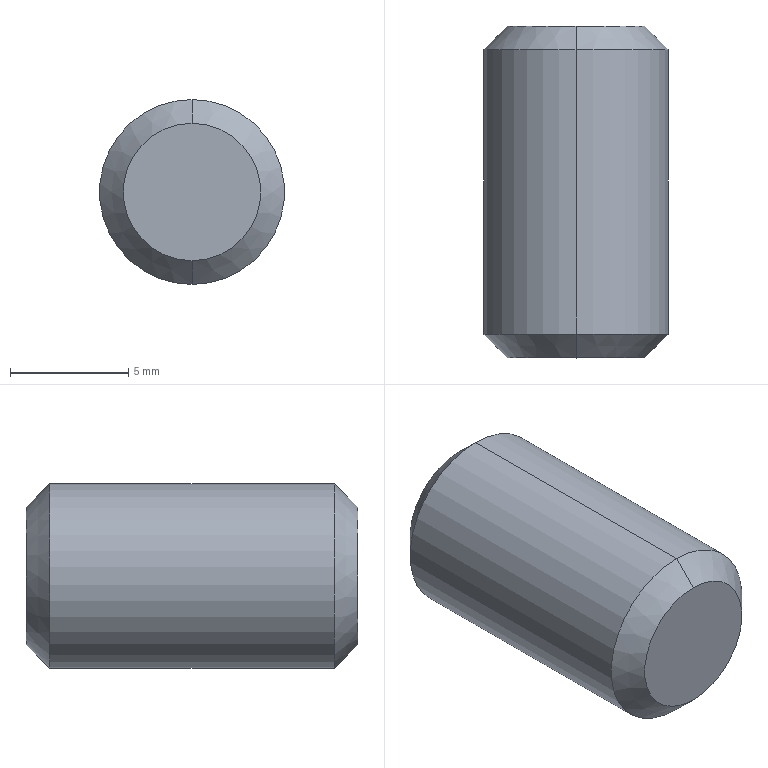Part | STEP file | Ngam kep 17 | 1 solid | 12 faces | box 7.8 x 14 x 7.8 mm | volume 557.349 mm3 | cone 6 | cylinder 4 | plane 2 | commonest cylinder face diameters 3.3 x2 7.8 x2
STEP:
#1=CARTESIAN_POINT('',(0.,0.,0.));
#2=DIRECTION('',(0.,0.,1.));
#3=DIRECTION('',(1.,0.,0.));
#4=AXIS2_PLACEMENT_3D('',#1,#2,#3);
#5=CARTESIAN_POINT('',(0.,14.,2.9));
#6=VERTEX_POINT('',#5);
#7=CARTESIAN_POINT('',(0.,14.,-2.9));
#8=VERTEX_POINT('',#7);
#9=CARTESIAN_POINT('',(0.,14.,0.));
#10=DIRECTION('',(0.,1.,0.));
#11=DIRECTION('',(0.,0.,1.));
#12=AXIS2_PLACEMENT_3D('',#9,#10,#11);
#13=CIRCLE('',#12,2.9);
#14=CARTESIAN_POINT('',(0.,14.,0.));
#15=DIRECTION('',(0.,-1.,0.));
#16=DIRECTION('',(0.,0.,-1.));
#17=AXIS2_PLACEMENT_3D('',#14,#15,#16);
#18=CONICAL_SURFACE('',#17,2.9,0.7854);
#19=CARTESIAN_POINT('',(3.142,0.));
#20=DIRECTION('',(-1.,0.));
#21=VECTOR('',#20,1.);
#22=LINE('',#19,#21);
#23=(GEOMETRIC_REPRESENTATION_CONTEXT(2)PARAMETRIC_REPRESENTATION_CONTEXT()REPRESENTATION_CONTEXT('',''));
#24=DEFINITIONAL_REPRESENTATION('',(#22),#23);
#25=PCURVE('',#18,#24);
#26=CARTESIAN_POINT('',(0.,14.,0.));
#27=DIRECTION('',(0.,1.,0.));
#28=DIRECTION('',(0.,0.,1.));
#29=AXIS2_PLACEMENT_3D('',#26,#27,#28);
#30=PLANE('',#29);
#31=CARTESIAN_POINT('',(0.,0.));
#32=DIRECTION('',(1.,0.));
#33=AXIS2_PLACEMENT_2D('',#31,#32);
#34=CIRCLE('',#33,2.9);
#35=(GEOMETRIC_REPRESENTATION_CONTEXT(2)PARAMETRIC_REPRESENTATION_CONTEXT()REPRESENTATION_CONTEXT('',''));
#36=DEFINITIONAL_REPRESENTATION('',(#34),#35);
#37=PCURVE('',#30,#36);
#38=SURFACE_CURVE('',#13,(#25,#37),.PCURVE_S1.);
#39=EDGE_CURVE('',#6,#8,#38,.T.);
#40=ORIENTED_EDGE('',*,*,#39,.F.);
#41=CARTESIAN_POINT('',(0.,13.,3.9));
#42=VERTEX_POINT('',#41);
#43=CARTESIAN_POINT('',(0.,14.,2.9));
#44=DIRECTION('',(0.,-0.7071,0.7071));
#45=VECTOR('',#44,1.);
#46=LINE('',#43,#45);
#47=CARTESIAN_POINT('',(3.142,0.));
#48=DIRECTION('',(0.,1.));
#49=VECTOR('',#48,1.);
#50=LINE('',#47,#49);
#51=(GEOMETRIC_REPRESENTATION_CONTEXT(2)PARAMETRIC_REPRESENTATION_CONTEXT()REPRESENTATION_CONTEXT('',''));
#52=DEFINITIONAL_REPRESENTATION('',(#50),#51);
#53=PCURVE('',#18,#52);
#54=CARTESIAN_POINT('',(0.,14.,0.));
#55=DIRECTION('',(0.,-1.,0.));
#56=DIRECTION('',(0.,0.,-1.));
#57=AXIS2_PLACEMENT_3D('',#54,#55,#56);
#58=CONICAL_SURFACE('',#57,2.9,0.7854);
#59=CARTESIAN_POINT('',(3.142,0.));
#60=DIRECTION('',(0.,1.));
#61=VECTOR('',#60,1.);
#62=LINE('',#59,#61);
#63=(GEOMETRIC_REPRESENTATION_CONTEXT(2)PARAMETRIC_REPRESENTATION_CONTEXT()REPRESENTATION_CONTEXT('',''));
#64=DEFINITIONAL_REPRESENTATION('',(#62),#63);
#65=PCURVE('',#58,#64);
#66=SURFACE_CURVE('',#46,(#53,#65),.PCURVE_S1.);
#67=EDGE_CURVE('',#6,#42,#66,.T.);
#68=ORIENTED_EDGE('',*,*,#67,.T.);
#69=CARTESIAN_POINT('',(0.,13.,-3.9));
#70=VERTEX_POINT('',#69);
#71=CARTESIAN_POINT('',(0.,13.,0.));
#72=DIRECTION('',(0.,-1.,0.));
#73=DIRECTION('',(0.,0.,1.));
#74=AXIS2_PLACEMENT_3D('',#71,#72,#73);
#75=CIRCLE('',#74,3.9);
#76=CARTESIAN_POINT('',(-3.142,1.));
#77=DIRECTION('',(1.,0.));
#78=VECTOR('',#77,1.);
#79=LINE('',#76,#78);
#80=(GEOMETRIC_REPRESENTATION_CONTEXT(2)PARAMETRIC_REPRESENTATION_CONTEXT()REPRESENTATION_CONTEXT('',''));
#81=DEFINITIONAL_REPRESENTATION('',(#79),#80);
#82=PCURVE('',#18,#81);
#83=CARTESIAN_POINT('',(0.,14.,0.));
#84=DIRECTION('',(0.,-1.,0.));
#85=DIRECTION('',(0.,0.,-1.));
#86=AXIS2_PLACEMENT_3D('',#83,#84,#85);
#87=CYLINDRICAL_SURFACE('',#86,3.9);
#88=CARTESIAN_POINT('',(-3.142,1.));
#89=DIRECTION('',(1.,0.));
#90=VECTOR('',#89,1.);
#91=LINE('',#88,#90);
#92=(GEOMETRIC_REPRESENTATION_CONTEXT(2)PARAMETRIC_REPRESENTATION_CONTEXT()REPRESENTATION_CONTEXT('',''));
#93=DEFINITIONAL_REPRESENTATION('',(#91),#92);
#94=PCURVE('',#87,#93);
#95=SURFACE_CURVE('',#75,(#82,#94),.PCURVE_S1.);
#96=EDGE_CURVE('',#70,#42,#95,.T.);
#97=ORIENTED_EDGE('',*,*,#96,.F.);
#98=CARTESIAN_POINT('',(0.,14.,-2.9));
#99=DIRECTION('',(0.,-0.7071,-0.7071));
#100=VECTOR('',#99,1.);
#101=LINE('',#98,#100);
#102=CARTESIAN_POINT('',(0.,0.));
#103=DIRECTION('',(0.,1.));
#104=VECTOR('',#103,1.);
#105=LINE('',#102,#104);
#106=(GEOMETRIC_REPRESENTATION_CONTEXT(2)PARAMETRIC_REPRESENTATION_CONTEXT()REPRESENTATION_CONTEXT('',''));
#107=DEFINITIONAL_REPRESENTATION('',(#105),#106);
#108=PCURVE('',#18,#107);
#109=CARTESIAN_POINT('',(6.283,0.));
#110=DIRECTION('',(0.,1.));
#111=VECTOR('',#110,1.);
#112=LINE('',#109,#111);
#113=(GEOMETRIC_REPRESENTATION_CONTEXT(2)PARAMETRIC_REPRESENTATION_CONTEXT()REPRESENTATION_CONTEXT('',''));
#114=DEFINITIONAL_REPRESENTATION('',(#112),#113);
#115=PCURVE('',#58,#114);
#116=SURFACE_CURVE('',#101,(#108,#115),.PCURVE_S1.);
#117=EDGE_CURVE('',#8,#70,#116,.T.);
#118=ORIENTED_EDGE('',*,*,#117,.F.);
#119=EDGE_LOOP('',(#40,#68,#97,#118));
#120=FACE_BOUND('',#119,.T.);
#121=ADVANCED_FACE('',(#120),#18,.T.);
#122=CARTESIAN_POINT('',(0.,0.,-2.9));
#123=VERTEX_POINT('',#122);
#124=CARTESIAN_POINT('',(0.,0.,2.9));
#125=VERTEX_POINT('',#124);
#126=CARTESIAN_POINT('',(0.,0.,0.));
#127=DIRECTION('',(0.,-1.,0.));
#128=DIRECTION('',(0.,0.,1.));
#129=AXIS2_PLACEMENT_3D('',#126,#127,#128);
#130=CIRCLE('',#129,2.9);
#131=CARTESIAN_POINT('',(0.,1.,0.));
#132=DIRECTION('',(0.,1.,0.));
#133=DIRECTION('',(0.,0.,1.));
#134=AXIS2_PLACEMENT_3D('',#131,#132,#133);
#135=CONICAL_SURFACE('',#134,3.9,0.7854);
#136=CARTESIAN_POINT('',(6.283,-1.));
#137=DIRECTION('',(-1.,0.));
#138=VECTOR('',#137,1.);
#139=LINE('',#136,#138);
#140=(GEOMETRIC_REPRESENTATION_CONTEXT(2)PARAMETRIC_REPRESENTATION_CONTEXT()REPRESENTATION_CONTEXT('',''));
#141=DEFINITIONAL_REPRESENTATION('',(#139),#140);
#142=PCURVE('',#135,#141);
#143=CARTESIAN_POINT('',(0.,0.,0.));
#144=DIRECTION('',(0.,1.,0.));
#145=DIRECTION('',(0.,0.,1.));
#146=AXIS2_PLACEMENT_3D('',#143,#144,#145);
#147=PLANE('',#146);
#148=CARTESIAN_POINT('',(2.9,0.));
#149=CARTESIAN_POINT('',(2.9,-5.023));
#150=CARTESIAN_POINT('',(-1.45,-2.511));
#151=CARTESIAN_POINT('',(-5.8,0.));
#152=CARTESIAN_POINT('',(-1.45,2.511));
#153=CARTESIAN_POINT('',(2.9,5.023));
#154=CARTESIAN_POINT('',(2.9,0.));
#155=(BOUNDED_CURVE()B_SPLINE_CURVE(2,(#148,#149,#150,#151,#152,#153,#154),.UNSPECIFIED.,.T.,.F.)B_SPLINE_CURVE_WITH_KNOTS((1,2,2,2,2,1),(-2.094,0.,2.094,4.189,6.283,8.378),.UNSPECIFIED.)CURVE()GEOMETRIC_REPRESENTATION_ITEM()RATIONAL_B_SPLINE_CURVE((1.,0.5,1.,0.5,1.,0.5,1.))REPRESENTATION_ITEM(''));
#156=(GEOMETRIC_REPRESENTATION_CONTEXT(2)PARAMETRIC_REPRESENTATION_CONTEXT()REPRESENTATION_CONTEXT('',''));
#157=DEFINITIONAL_REPRESENTATION('',(#155),#156);
#158=PCURVE('',#147,#157);
#159=SURFACE_CURVE('',#130,(#142,#158),.PCURVE_S1.);
#160=EDGE_CURVE('',#123,#125,#159,.T.);
#161=ORIENTED_EDGE('',*,*,#160,.F.);
#162=CARTESIAN_POINT('',(0.,1.,-3.9));
#163=VERTEX_POINT('',#162);
#164=CARTESIAN_POINT('',(0.,1.,-3.9));
#165=DIRECTION('',(0.,0.7071,-0.7071));
#166=VECTOR('',#165,1.);
#167=LINE('',#164,#166);
#168=CARTESIAN_POINT('',(3.142,0.));
#169=DIRECTION('',(0.,1.));
#170=VECTOR('',#169,1.);
#171=LINE('',#168,#170);
#172=(GEOMETRIC_REPRESENTATION_CONTEXT(2)PARAMETRIC_REPRESENTATION_CONTEXT()REPRESENTATION_CONTEXT('',''));
#173=DEFINITIONAL_REPRESENTATION('',(#171),#172);
#174=PCURVE('',#135,#173);
#175=CARTESIAN_POINT('',(0.,1.,0.));
#176=DIRECTION('',(0.,1.,0.));
#177=DIRECTION('',(0.,0.,1.));
#178=AXIS2_PLACEMENT_3D('',#175,#176,#177);
#179=CONICAL_SURFACE('',#178,3.9,0.7854);
#180=CARTESIAN_POINT('',(3.142,0.));
#181=DIRECTION('',(0.,1.));
#182=VECTOR('',#181,1.);
#183=LINE('',#180,#182);
#184=(GEOMETRIC_REPRESENTATION_CONTEXT(2)PARAMETRIC_REPRESENTATION_CONTEXT()REPRESENTATION_CONTEXT('',''));
#185=DEFINITIONAL_REPRESENTATION('',(#183),#184);
#186=PCURVE('',#179,#185);
#187=SURFACE_CURVE('',#167,(#174,#186),.PCURVE_S1.);
#188=EDGE_CURVE('',#123,#163,#187,.T.);
#189=ORIENTED_EDGE('',*,*,#188,.T.);
#190=CARTESIAN_POINT('',(0.,1.,3.9));
#191=VERTEX_POINT('',#190);
#192=CARTESIAN_POINT('',(0.,1.,0.));
#193=DIRECTION('',(0.,1.,0.));
#194=DIRECTION('',(0.,0.,1.));
#195=AXIS2_PLACEMENT_3D('',#192,#193,#194);
#196=CIRCLE('',#195,3.9);
#197=CARTESIAN_POINT('',(0.,0.));
#198=DIRECTION('',(1.,0.));
#199=VECTOR('',#198,1.);
#200=LINE('',#197,#199);
#201=(GEOMETRIC_REPRESENTATION_CONTEXT(2)PARAMETRIC_REPRESENTATION_CONTEXT()REPRESENTATION_CONTEXT('',''));
#202=DEFINITIONAL_REPRESENTATION('',(#200),#201);
#203=PCURVE('',#135,#202);
#204=CARTESIAN_POINT('',(3.142,13.));
#205=DIRECTION('',(-1.,0.));
#206=VECTOR('',#205,1.);
#207=LINE('',#204,#206);
#208=(GEOMETRIC_REPRESENTATION_CONTEXT(2)PARAMETRIC_REPRESENTATION_CONTEXT()REPRESENTATION_CONTEXT('',''));
#209=DEFINITIONAL_REPRESENTATION('',(#207),#208);
#210=PCURVE('',#87,#209);
#211=SURFACE_CURVE('',#196,(#203,#210),.PCURVE_S1.);
#212=EDGE_CURVE('',#191,#163,#211,.T.);
#213=ORIENTED_EDGE('',*,*,#212,.F.);
#214=CARTESIAN_POINT('',(0.,1.,3.9));
#215=DIRECTION('',(0.,0.7071,0.7071));
#216=VECTOR('',#215,1.);
#217=LINE('',#214,#216);
#218=CARTESIAN_POINT('',(0.,0.));
#219=DIRECTION('',(0.,1.));
#220=VECTOR('',#219,1.);
#221=LINE('',#218,#220);
#222=(GEOMETRIC_REPRESENTATION_CONTEXT(2)PARAMETRIC_REPRESENTATION_CONTEXT()REPRESENTATION_CONTEXT('',''));
#223=DEFINITIONAL_REPRESENTATION('',(#221),#222);
#224=PCURVE('',#135,#223);
#225=CARTESIAN_POINT('',(6.283,0.));
#226=DIRECTION('',(0.,1.));
#227=VECTOR('',#226,1.);
#228=LINE('',#225,#227);
#229=(GEOMETRIC_REPRESENTATION_CONTEXT(2)PARAMETRIC_REPRESENTATION_CONTEXT()REPRESENTATION_CONTEXT('',''));
#230=DEFINITIONAL_REPRESENTATION('',(#228),#229);
#231=PCURVE('',#179,#230);
#232=SURFACE_CURVE('',#217,(#224,#231),.PCURVE_S1.);
#233=EDGE_CURVE('',#125,#191,#232,.T.);
#234=ORIENTED_EDGE('',*,*,#233,.F.);
#235=EDGE_LOOP('',(#161,#189,#213,#234));
#236=FACE_BOUND('',#235,.T.);
#237=ADVANCED_FACE('',(#236),#135,.T.);
#238=CARTESIAN_POINT('',(0.,3.9,1.65));
#239=VERTEX_POINT('',#238);
#240=CARTESIAN_POINT('',(0.,14.,1.65));
#241=VERTEX_POINT('',#240);
#242=CARTESIAN_POINT('',(0.,14.,1.65));
#243=DIRECTION('',(0.,1.,0.));
#244=VECTOR('',#243,1.);
#245=LINE('',#242,#244);
#246=CARTESIAN_POINT('',(0.,14.,0.));
#247=DIRECTION('',(0.,1.,0.));
#248=DIRECTION('',(0.,0.,1.));
#249=AXIS2_PLACEMENT_3D('',#246,#247,#248);
#250=CYLINDRICAL_SURFACE('',#249,1.65);
#251=CARTESIAN_POINT('',(6.283,0.));
#252=DIRECTION('',(0.,1.));
#253=VECTOR('',#252,1.);
#254=LINE('',#251,#253);
#255=(GEOMETRIC_REPRESENTATION_CONTEXT(2)PARAMETRIC_REPRESENTATION_CONTEXT()REPRESENTATION_CONTEXT('',''));
#256=DEFINITIONAL_REPRESENTATION('',(#254),#255);
#257=PCURVE('',#250,#256);
#258=CARTESIAN_POINT('',(0.,14.,0.));
#259=DIRECTION('',(0.,1.,0.));
#260=DIRECTION('',(0.,0.,1.));
#261=AXIS2_PLACEMENT_3D('',#258,#259,#260);
#262=CYLINDRICAL_SURFACE('',#261,1.65);
#263=CARTESIAN_POINT('',(0.,0.));
#264=DIRECTION('',(0.,1.));
#265=VECTOR('',#264,1.);
#266=LINE('',#263,#265);
#267=(GEOMETRIC_REPRESENTATION_CONTEXT(2)PARAMETRIC_REPRESENTATION_CONTEXT()REPRESENTATION_CONTEXT('',''));
#268=DEFINITIONAL_REPRESENTATION('',(#266),#267);
#269=PCURVE('',#262,#268);
#270=SURFACE_CURVE('',#245,(#257,#269),.PCURVE_S1.);
#271=EDGE_CURVE('',#239,#241,#270,.T.);
#272=ORIENTED_EDGE('',*,*,#271,.T.);
#273=CARTESIAN_POINT('',(0.,14.,-1.65));
#274=VERTEX_POINT('',#273);
#275=CARTESIAN_POINT('',(0.,14.,0.));
#276=DIRECTION('',(0.,1.,0.));
#277=DIRECTION('',(0.,0.,1.));
#278=AXIS2_PLACEMENT_3D('',#275,#276,#277);
#279=CIRCLE('',#278,1.65);
#280=CARTESIAN_POINT('',(0.,0.));
#281=DIRECTION('',(1.,0.));
#282=VECTOR('',#281,1.);
#283=LINE('',#280,#282);
#284=(GEOMETRIC_REPRESENTATION_CONTEXT(2)PARAMETRIC_REPRESENTATION_CONTEXT()REPRESENTATION_CONTEXT('',''));
#285=DEFINITIONAL_REPRESENTATION('',(#283),#284);
#286=PCURVE('',#250,#285);
#287=CARTESIAN_POINT('',(0.,0.));
#288=DIRECTION('',(1.,0.));
#289=AXIS2_PLACEMENT_2D('',#287,#288);
#290=CIRCLE('',#289,1.65);
#291=(GEOMETRIC_REPRESENTATION_CONTEXT(2)PARAMETRIC_REPRESENTATION_CONTEXT()REPRESENTATION_CONTEXT('',''));
#292=DEFINITIONAL_REPRESENTATION('',(#290),#291);
#293=PCURVE('',#30,#292);
#294=SURFACE_CURVE('',#279,(#286,#293),.PCURVE_S1.);
#295=EDGE_CURVE('',#274,#241,#294,.T.);
#296=ORIENTED_EDGE('',*,*,#295,.F.);
#297=CARTESIAN_POINT('',(0.,3.9,-1.65));
#298=VERTEX_POINT('',#297);
#299=CARTESIAN_POINT('',(0.,14.,-1.65));
#300=DIRECTION('',(0.,1.,0.));
#301=VECTOR('',#300,1.);
#302=LINE('',#299,#301);
#303=CARTESIAN_POINT('',(3.142,0.));
#304=DIRECTION('',(0.,1.));
#305=VECTOR('',#304,1.);
#306=LINE('',#303,#305);
#307=(GEOMETRIC_REPRESENTATION_CONTEXT(2)PARAMETRIC_REPRESENTATION_CONTEXT()REPRESENTATION_CONTEXT('',''));
#308=DEFINITIONAL_REPRESENTATION('',(#306),#307);
#309=PCURVE('',#250,#308);
#310=CARTESIAN_POINT('',(3.142,0.));
#311=DIRECTION('',(0.,1.));
#312=VECTOR('',#311,1.);
#313=LINE('',#310,#312);
#314=(GEOMETRIC_REPRESENTATION_CONTEXT(2)PARAMETRIC_REPRESENTATION_CONTEXT()REPRESENTATION_CONTEXT('',''));
#315=DEFINITIONAL_REPRESENTATION('',(#313),#314);
#316=PCURVE('',#262,#315);
#317=SURFACE_CURVE('',#302,(#309,#316),.PCURVE_S1.);
#318=EDGE_CURVE('',#298,#274,#317,.T.);
#319=ORIENTED_EDGE('',*,*,#318,.F.);
#320=CARTESIAN_POINT('',(0.,3.9,0.));
#321=DIRECTION('',(0.,1.,0.));
#322=DIRECTION('',(0.,0.,1.));
#323=AXIS2_PLACEMENT_3D('',#320,#321,#322);
#324=CIRCLE('',#323,1.65);
#325=CARTESIAN_POINT('',(0.,-10.1));
#326=DIRECTION('',(1.,0.));
#327=VECTOR('',#326,1.);
#328=LINE('',#325,#327);
#329=(GEOMETRIC_REPRESENTATION_CONTEXT(2)PARAMETRIC_REPRESENTATION_CONTEXT()REPRESENTATION_CONTEXT('',''));
#330=DEFINITIONAL_REPRESENTATION('',(#328),#329);
#331=PCURVE('',#250,#330);
#332=CARTESIAN_POINT('',(0.,3.9,0.));
#333=DIRECTION('',(0.,1.,0.));
#334=DIRECTION('',(0.,0.,1.));
#335=AXIS2_PLACEMENT_3D('',#332,#333,#334);
#336=CONICAL_SURFACE('',#335,1.65,1.03);
#337=CARTESIAN_POINT('',(0.,0.));
#338=DIRECTION('',(1.,0.));
#339=VECTOR('',#338,1.);
#340=LINE('',#337,#339);
#341=(GEOMETRIC_REPRESENTATION_CONTEXT(2)PARAMETRIC_REPRESENTATION_CONTEXT()REPRESENTATION_CONTEXT('',''));
#342=DEFINITIONAL_REPRESENTATION('',(#340),#341);
#343=PCURVE('',#336,#342);
#344=SURFACE_CURVE('',#324,(#331,#343),.PCURVE_S1.);
#345=EDGE_CURVE('',#298,#239,#344,.T.);
#346=ORIENTED_EDGE('',*,*,#345,.T.);
#347=EDGE_LOOP('',(#272,#296,#319,#346));
#348=FACE_BOUND('',#347,.F.);
#349=ADVANCED_FACE('',(#348),#250,.F.);
#350=ORIENTED_EDGE('',*,*,#345,.F.);
#351=CARTESIAN_POINT('',(0.,2.909,0.));
#352=VERTEX_POINT('',#351);
#353=CARTESIAN_POINT('',(0.,3.9,-1.65));
#354=DIRECTION('',(0.,0.515,-0.8572));
#355=VECTOR('',#354,1.);
#356=LINE('',#353,#355);
#357=CARTESIAN_POINT('',(3.142,0.));
#358=DIRECTION('',(0.,1.));
#359=VECTOR('',#358,1.);
#360=LINE('',#357,#359);
#361=(GEOMETRIC_REPRESENTATION_CONTEXT(2)PARAMETRIC_REPRESENTATION_CONTEXT()REPRESENTATION_CONTEXT('',''));
#362=DEFINITIONAL_REPRESENTATION('',(#360),#361);
#363=PCURVE('',#336,#362);
#364=CARTESIAN_POINT('',(0.,3.9,0.));
#365=DIRECTION('',(0.,1.,0.));
#366=DIRECTION('',(0.,0.,1.));
#367=AXIS2_PLACEMENT_3D('',#364,#365,#366);
#368=CONICAL_SURFACE('',#367,1.65,1.03);
#369=CARTESIAN_POINT('',(3.142,0.));
#370=DIRECTION('',(0.,1.));
#371=VECTOR('',#370,1.);
#372=LINE('',#369,#371);
#373=(GEOMETRIC_REPRESENTATION_CONTEXT(2)PARAMETRIC_REPRESENTATION_CONTEXT()REPRESENTATION_CONTEXT('',''));
#374=DEFINITIONAL_REPRESENTATION('',(#372),#373);
#375=PCURVE('',#368,#374);
#376=SURFACE_CURVE('',#356,(#363,#375),.PCURVE_S1.);
#377=EDGE_CURVE('',#352,#298,#376,.T.);
#378=ORIENTED_EDGE('',*,*,#377,.F.);
#379=CARTESIAN_POINT('',(0.,3.9,1.65));
#380=DIRECTION('',(0.,0.515,0.8572));
#381=VECTOR('',#380,1.);
#382=LINE('',#379,#381);
#383=CARTESIAN_POINT('',(6.283,0.));
#384=DIRECTION('',(0.,1.));
#385=VECTOR('',#384,1.);
#386=LINE('',#383,#385);
#387=(GEOMETRIC_REPRESENTATION_CONTEXT(2)PARAMETRIC_REPRESENTATION_CONTEXT()REPRESENTATION_CONTEXT('',''));
#388=DEFINITIONAL_REPRESENTATION('',(#386),#387);
#389=PCURVE('',#336,#388);
#390=CARTESIAN_POINT('',(0.,0.));
#391=DIRECTION('',(0.,1.));
#392=VECTOR('',#391,1.);
#393=LINE('',#390,#392);
#394=(GEOMETRIC_REPRESENTATION_CONTEXT(2)PARAMETRIC_REPRESENTATION_CONTEXT()REPRESENTATION_CONTEXT('',''));
#395=DEFINITIONAL_REPRESENTATION('',(#393),#394);
#396=PCURVE('',#368,#395);
#397=SURFACE_CURVE('',#382,(#389,#396),.PCURVE_S1.);
#398=EDGE_CURVE('',#352,#239,#397,.T.);
#399=ORIENTED_EDGE('',*,*,#398,.T.);
#400=EDGE_LOOP('',(#350,#378,#399));
#401=FACE_BOUND('',#400,.F.);
#402=ADVANCED_FACE('',(#401),#336,.F.);
#403=ORIENTED_EDGE('',*,*,#96,.T.);
#404=CARTESIAN_POINT('',(0.,14.,3.9));
#405=DIRECTION('',(0.,-1.,0.));
#406=VECTOR('',#405,1.);
#407=LINE('',#404,#406);
#408=CARTESIAN_POINT('',(3.142,0.));
#409=DIRECTION('',(0.,1.));
#410=VECTOR('',#409,1.);
#411=LINE('',#408,#410);
#412=(GEOMETRIC_REPRESENTATION_CONTEXT(2)PARAMETRIC_REPRESENTATION_CONTEXT()REPRESENTATION_CONTEXT('',''));
#413=DEFINITIONAL_REPRESENTATION('',(#411),#412);
#414=PCURVE('',#87,#413);
#415=CARTESIAN_POINT('',(0.,14.,0.));
#416=DIRECTION('',(0.,-1.,0.));
#417=DIRECTION('',(0.,0.,-1.));
#418=AXIS2_PLACEMENT_3D('',#415,#416,#417);
#419=CYLINDRICAL_SURFACE('',#418,3.9);
#420=CARTESIAN_POINT('',(3.142,0.));
#421=DIRECTION('',(0.,1.));
#422=VECTOR('',#421,1.);
#423=LINE('',#420,#422);
#424=(GEOMETRIC_REPRESENTATION_CONTEXT(2)PARAMETRIC_REPRESENTATION_CONTEXT()REPRESENTATION_CONTEXT('',''));
#425=DEFINITIONAL_REPRESENTATION('',(#423),#424);
#426=PCURVE('',#419,#425);
#427=SURFACE_CURVE('',#407,(#414,#426),.PCURVE_S1.);
#428=EDGE_CURVE('',#42,#191,#427,.T.);
#429=ORIENTED_EDGE('',*,*,#428,.T.);
#430=ORIENTED_EDGE('',*,*,#212,.T.);
#431=CARTESIAN_POINT('',(0.,14.,-3.9));
#432=DIRECTION('',(0.,-1.,0.));
#433=VECTOR('',#432,1.);
#434=LINE('',#431,#433);
#435=CARTESIAN_POINT('',(0.,0.));
#436=DIRECTION('',(0.,1.));
#437=VECTOR('',#436,1.);
#438=LINE('',#435,#437);
#439=(GEOMETRIC_REPRESENTATION_CONTEXT(2)PARAMETRIC_REPRESENTATION_CONTEXT()REPRESENTATION_CONTEXT('',''));
#440=DEFINITIONAL_REPRESENTATION('',(#438),#439);
#441=PCURVE('',#87,#440);
#442=CARTESIAN_POINT('',(6.283,0.));
#443=DIRECTION('',(0.,1.));
#444=VECTOR('',#443,1.);
#445=LINE('',#442,#444);
#446=(GEOMETRIC_REPRESENTATION_CONTEXT(2)PARAMETRIC_REPRESENTATION_CONTEXT()REPRESENTATION_CONTEXT('',''));
#447=DEFINITIONAL_REPRESENTATION('',(#445),#446);
#448=PCURVE('',#419,#447);
#449=SURFACE_CURVE('',#434,(#441,#448),.PCURVE_S1.);
#450=EDGE_CURVE('',#70,#163,#449,.T.);
#451=ORIENTED_EDGE('',*,*,#450,.F.);
#452=EDGE_LOOP('',(#403,#429,#430,#451));
#453=FACE_BOUND('',#452,.T.);
#454=ADVANCED_FACE('',(#453),#87,.T.);
#455=ORIENTED_EDGE('',*,*,#428,.F.);
#456=CARTESIAN_POINT('',(0.,13.,0.));
#457=DIRECTION('',(0.,-1.,0.));
#458=DIRECTION('',(0.,0.,1.));
#459=AXIS2_PLACEMENT_3D('',#456,#457,#458);
#460=CIRCLE('',#459,3.9);
#461=CARTESIAN_POINT('',(3.142,1.));
#462=DIRECTION('',(1.,0.));
#463=VECTOR('',#462,1.);
#464=LINE('',#461,#463);
#465=(GEOMETRIC_REPRESENTATION_CONTEXT(2)PARAMETRIC_REPRESENTATION_CONTEXT()REPRESENTATION_CONTEXT('',''));
#466=DEFINITIONAL_REPRESENTATION('',(#464),#465);
#467=PCURVE('',#419,#466);
#468=CARTESIAN_POINT('',(3.142,1.));
#469=DIRECTION('',(1.,0.));
#470=VECTOR('',#469,1.);
#471=LINE('',#468,#470);
#472=(GEOMETRIC_REPRESENTATION_CONTEXT(2)PARAMETRIC_REPRESENTATION_CONTEXT()REPRESENTATION_CONTEXT('',''));
#473=DEFINITIONAL_REPRESENTATION('',(#471),#472);
#474=PCURVE('',#58,#473);
#475=SURFACE_CURVE('',#460,(#467,#474),.PCURVE_S1.);
#476=EDGE_CURVE('',#42,#70,#475,.T.);
#477=ORIENTED_EDGE('',*,*,#476,.T.);
#478=ORIENTED_EDGE('',*,*,#450,.T.);
#479=CARTESIAN_POINT('',(0.,1.,0.));
#480=DIRECTION('',(0.,1.,0.));
#481=DIRECTION('',(0.,0.,1.));
#482=AXIS2_PLACEMENT_3D('',#479,#480,#481);
#483=CIRCLE('',#482,3.9);
#484=CARTESIAN_POINT('',(9.425,13.));
#485=DIRECTION('',(-1.,0.));
#486=VECTOR('',#485,1.);
#487=LINE('',#484,#486);
#488=(GEOMETRIC_REPRESENTATION_CONTEXT(2)PARAMETRIC_REPRESENTATION_CONTEXT()REPRESENTATION_CONTEXT('',''));
#489=DEFINITIONAL_REPRESENTATION('',(#487),#488);
#490=PCURVE('',#419,#489);
#491=CARTESIAN_POINT('',(0.,0.));
#492=DIRECTION('',(1.,0.));
#493=VECTOR('',#492,1.);
#494=LINE('',#491,#493);
#495=(GEOMETRIC_REPRESENTATION_CONTEXT(2)PARAMETRIC_REPRESENTATION_CONTEXT()REPRESENTATION_CONTEXT('',''));
#496=DEFINITIONAL_REPRESENTATION('',(#494),#495);
#497=PCURVE('',#179,#496);
#498=SURFACE_CURVE('',#483,(#490,#497),.PCURVE_S1.);
#499=EDGE_CURVE('',#163,#191,#498,.T.);
#500=ORIENTED_EDGE('',*,*,#499,.T.);
#501=EDGE_LOOP('',(#455,#477,#478,#500));
#502=FACE_BOUND('',#501,.T.);
#503=ADVANCED_FACE('',(#502),#419,.T.);
#504=CARTESIAN_POINT('',(0.,14.,0.));
#505=DIRECTION('',(0.,1.,0.));
#506=DIRECTION('',(0.,0.,1.));
#507=AXIS2_PLACEMENT_3D('',#504,#505,#506);
#508=CIRCLE('',#507,2.9);
#509=CARTESIAN_POINT('',(0.,0.));
#510=DIRECTION('',(1.,0.));
#511=AXIS2_PLACEMENT_2D('',#509,#510);
#512=CIRCLE('',#511,2.9);
#513=(GEOMETRIC_REPRESENTATION_CONTEXT(2)PARAMETRIC_REPRESENTATION_CONTEXT()REPRESENTATION_CONTEXT('',''));
#514=DEFINITIONAL_REPRESENTATION('',(#512),#513);
#515=PCURVE('',#30,#514);
#516=CARTESIAN_POINT('',(9.425,0.));
#517=DIRECTION('',(-1.,0.));
#518=VECTOR('',#517,1.);
#519=LINE('',#516,#518);
#520=(GEOMETRIC_REPRESENTATION_CONTEXT(2)PARAMETRIC_REPRESENTATION_CONTEXT()REPRESENTATION_CONTEXT('',''));
#521=DEFINITIONAL_REPRESENTATION('',(#519),#520);
#522=PCURVE('',#58,#521);
#523=SURFACE_CURVE('',#508,(#515,#522),.PCURVE_S1.);
#524=EDGE_CURVE('',#8,#6,#523,.T.);
#525=ORIENTED_EDGE('',*,*,#524,.T.);
#526=ORIENTED_EDGE('',*,*,#39,.T.);
#527=EDGE_LOOP('',(#525,#526));
#528=FACE_BOUND('',#527,.T.);
#529=CARTESIAN_POINT('',(0.,14.,0.));
#530=DIRECTION('',(0.,1.,0.));
#531=DIRECTION('',(0.,0.,1.));
#532=AXIS2_PLACEMENT_3D('',#529,#530,#531);
#533=CIRCLE('',#532,1.65);
#534=CARTESIAN_POINT('',(0.,0.));
#535=DIRECTION('',(1.,0.));
#536=AXIS2_PLACEMENT_2D('',#534,#535);
#537=CIRCLE('',#536,1.65);
#538=(GEOMETRIC_REPRESENTATION_CONTEXT(2)PARAMETRIC_REPRESENTATION_CONTEXT()REPRESENTATION_CONTEXT('',''));
#539=DEFINITIONAL_REPRESENTATION('',(#537),#538);
#540=PCURVE('',#30,#539);
#541=CARTESIAN_POINT('',(0.,0.));
#542=DIRECTION('',(1.,0.));
#543=VECTOR('',#542,1.);
#544=LINE('',#541,#543);
#545=(GEOMETRIC_REPRESENTATION_CONTEXT(2)PARAMETRIC_REPRESENTATION_CONTEXT()REPRESENTATION_CONTEXT('',''));
#546=DEFINITIONAL_REPRESENTATION('',(#544),#545);
#547=PCURVE('',#262,#546);
#548=SURFACE_CURVE('',#533,(#540,#547),.PCURVE_S1.);
#549=EDGE_CURVE('',#241,#274,#548,.T.);
#550=ORIENTED_EDGE('',*,*,#549,.F.);
#551=ORIENTED_EDGE('',*,*,#295,.F.);
#552=EDGE_LOOP('',(#550,#551));
#553=FACE_BOUND('',#552,.T.);
#554=ADVANCED_FACE('',(#528,#553),#30,.T.);
#555=CARTESIAN_POINT('',(0.,0.,0.));
#556=DIRECTION('',(0.,-1.,0.));
#557=DIRECTION('',(0.,0.,1.));
#558=AXIS2_PLACEMENT_3D('',#555,#556,#557);
#559=CIRCLE('',#558,2.9);
#560=CARTESIAN_POINT('',(2.9,0.));
#561=CARTESIAN_POINT('',(2.9,-5.023));
#562=CARTESIAN_POINT('',(-1.45,-2.511));
#563=CARTESIAN_POINT('',(-5.8,0.));
#564=CARTESIAN_POINT('',(-1.45,2.511));
#565=CARTESIAN_POINT('',(2.9,5.023));
#566=CARTESIAN_POINT('',(2.9,0.));
#567=(BOUNDED_CURVE()B_SPLINE_CURVE(2,(#560,#561,#562,#563,#564,#565,#566),.UNSPECIFIED.,.T.,.F.)B_SPLINE_CURVE_WITH_KNOTS((1,2,2,2,2,1),(-2.094,0.,2.094,4.189,6.283,8.378),.UNSPECIFIED.)CURVE()GEOMETRIC_REPRESENTATION_ITEM()RATIONAL_B_SPLINE_CURVE((1.,0.5,1.,0.5,1.,0.5,1.))REPRESENTATION_ITEM(''));
#568=(GEOMETRIC_REPRESENTATION_CONTEXT(2)PARAMETRIC_REPRESENTATION_CONTEXT()REPRESENTATION_CONTEXT('',''));
#569=DEFINITIONAL_REPRESENTATION('',(#567),#568);
#570=PCURVE('',#147,#569);
#571=CARTESIAN_POINT('',(6.283,-1.));
#572=DIRECTION('',(-1.,0.));
#573=VECTOR('',#572,1.);
#574=LINE('',#571,#573);
#575=(GEOMETRIC_REPRESENTATION_CONTEXT(2)PARAMETRIC_REPRESENTATION_CONTEXT()REPRESENTATION_CONTEXT('',''));
#576=DEFINITIONAL_REPRESENTATION('',(#574),#575);
#577=PCURVE('',#179,#576);
#578=SURFACE_CURVE('',#559,(#570,#577),.PCURVE_S1.);
#579=EDGE_CURVE('',#125,#123,#578,.T.);
#580=ORIENTED_EDGE('',*,*,#579,.T.);
#581=ORIENTED_EDGE('',*,*,#160,.T.);
#582=EDGE_LOOP('',(#580,#581));
#583=FACE_BOUND('',#582,.T.);
#584=ADVANCED_FACE('',(#583),#147,.F.);
#585=CARTESIAN_POINT('',(0.,3.9,0.));
#586=DIRECTION('',(0.,1.,0.));
#587=DIRECTION('',(0.,0.,1.));
#588=AXIS2_PLACEMENT_3D('',#585,#586,#587);
#589=CIRCLE('',#588,1.65);
#590=CARTESIAN_POINT('',(0.,0.));
#591=DIRECTION('',(1.,0.));
#592=VECTOR('',#591,1.);
#593=LINE('',#590,#592);
#594=(GEOMETRIC_REPRESENTATION_CONTEXT(2)PARAMETRIC_REPRESENTATION_CONTEXT()REPRESENTATION_CONTEXT('',''));
#595=DEFINITIONAL_REPRESENTATION('',(#593),#594);
#596=PCURVE('',#368,#595);
#597=CARTESIAN_POINT('',(0.,-10.1));
#598=DIRECTION('',(1.,0.));
#599=VECTOR('',#598,1.);
#600=LINE('',#597,#599);
#601=(GEOMETRIC_REPRESENTATION_CONTEXT(2)PARAMETRIC_REPRESENTATION_CONTEXT()REPRESENTATION_CONTEXT('',''));
#602=DEFINITIONAL_REPRESENTATION('',(#600),#601);
#603=PCURVE('',#262,#602);
#604=SURFACE_CURVE('',#589,(#596,#603),.PCURVE_S1.);
#605=EDGE_CURVE('',#239,#298,#604,.T.);
#606=ORIENTED_EDGE('',*,*,#605,.F.);
#607=ORIENTED_EDGE('',*,*,#398,.F.);
#608=ORIENTED_EDGE('',*,*,#377,.T.);
#609=EDGE_LOOP('',(#606,#607,#608));
#610=FACE_BOUND('',#609,.F.);
#611=ADVANCED_FACE('',(#610),#368,.F.);
#612=ORIENTED_EDGE('',*,*,#549,.F.);
#613=ORIENTED_EDGE('',*,*,#271,.F.);
#614=ORIENTED_EDGE('',*,*,#605,.T.);
#615=ORIENTED_EDGE('',*,*,#318,.T.);
#616=EDGE_LOOP('',(#612,#613,#614,#615));
#617=FACE_BOUND('',#616,.F.);
#618=ADVANCED_FACE('',(#617),#262,.F.);
#619=ORIENTED_EDGE('',*,*,#188,.F.);
#620=ORIENTED_EDGE('',*,*,#579,.F.);
#621=ORIENTED_EDGE('',*,*,#233,.T.);
#622=ORIENTED_EDGE('',*,*,#499,.F.);
#623=EDGE_LOOP('',(#619,#620,#621,#622));
#624=FACE_BOUND('',#623,.T.);
#625=ADVANCED_FACE('',(#624),#179,.T.);
#626=ORIENTED_EDGE('',*,*,#67,.F.);
#627=ORIENTED_EDGE('',*,*,#524,.F.);
#628=ORIENTED_EDGE('',*,*,#117,.T.);
#629=ORIENTED_EDGE('',*,*,#476,.F.);
#630=EDGE_LOOP('',(#626,#627,#628,#629));
#631=FACE_BOUND('',#630,.T.);
#632=ADVANCED_FACE('',(#631),#58,.T.);
#633=CLOSED_SHELL('',(#121,#237,#349,#402,#454,#503,#554,#584,#611,#618,#625,#632));
#634=MANIFOLD_SOLID_BREP('',#633);
#635=(LENGTH_UNIT()NAMED_UNIT(*)SI_UNIT(.MILLI.,.METRE.));
#636=UNCERTAINTY_MEASURE_WITH_UNIT(LENGTH_MEASURE(0.0000001),#635,'','');
#637=(NAMED_UNIT(*)PLANE_ANGLE_UNIT()SI_UNIT($,.RADIAN.));
#638=(NAMED_UNIT(*)SI_UNIT($,.STERADIAN.)SOLID_ANGLE_UNIT());
#639=(GEOMETRIC_REPRESENTATION_CONTEXT(3)GLOBAL_UNCERTAINTY_ASSIGNED_CONTEXT((#636))GLOBAL_UNIT_ASSIGNED_CONTEXT((#635,#637,#638))REPRESENTATION_CONTEXT('',''));
#640=ADVANCED_BREP_SHAPE_REPRESENTATION('',(#4,#634),#639);